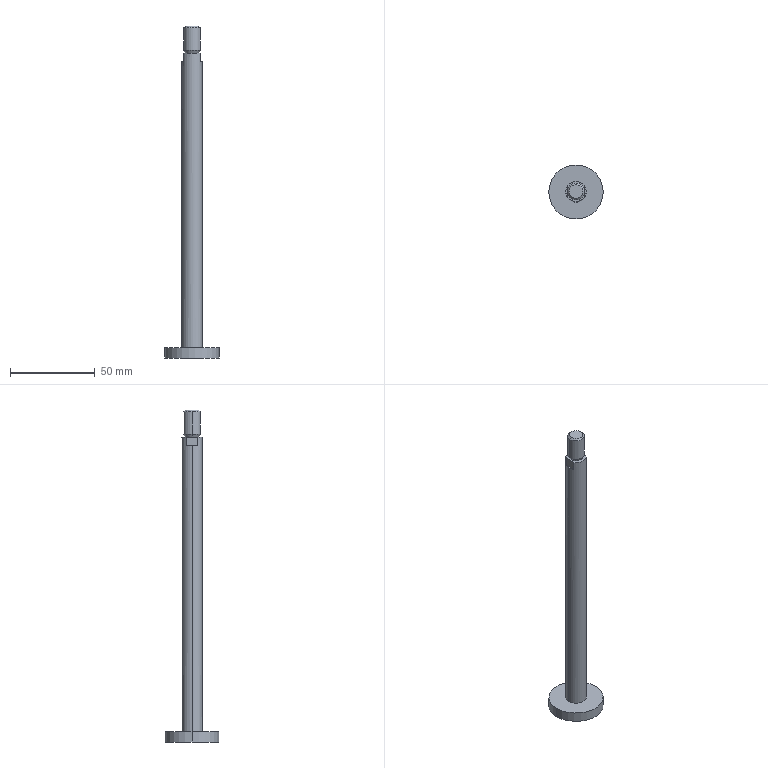Part | STEP file | 1 solid | 18 faces | box 32 x 32 x 195.5 mm | volume 25619 mm3 | plane 8 | cylinder 6 | cone 4 | commonest cylinder face diameters 10 x2 12 x2 32 x2
STEP:
#1=CARTESIAN_POINT('',(0.,0.,0.));
#2=DIRECTION('',(0.,0.,1.));
#3=DIRECTION('',(1.,0.,0.));
#4=AXIS2_PLACEMENT_3D('',#1,#2,#3);
#5=CARTESIAN_POINT('',(16.,0.,-158.5));
#6=VERTEX_POINT('',#5);
#7=CARTESIAN_POINT('',(-16.,0.,-158.5));
#8=VERTEX_POINT('',#7);
#9=CARTESIAN_POINT('',(0.,0.,-158.5));
#10=DIRECTION('',(0.,0.,1.));
#11=DIRECTION('',(1.,0.,0.));
#12=AXIS2_PLACEMENT_3D('',#9,#10,#11);
#13=CIRCLE('',#12,16.);
#14=CARTESIAN_POINT('',(0.,0.,-158.5));
#15=DIRECTION('',(0.,0.,1.));
#16=DIRECTION('',(1.,0.,0.));
#17=AXIS2_PLACEMENT_3D('',#14,#15,#16);
#18=CYLINDRICAL_SURFACE('',#17,16.);
#19=CARTESIAN_POINT('',(0.,0.));
#20=DIRECTION('',(1.,0.));
#21=VECTOR('',#20,1.);
#22=LINE('',#19,#21);
#23=(GEOMETRIC_REPRESENTATION_CONTEXT(2)PARAMETRIC_REPRESENTATION_CONTEXT()REPRESENTATION_CONTEXT('',''));
#24=DEFINITIONAL_REPRESENTATION('',(#22),#23);
#25=PCURVE('',#18,#24);
#26=CARTESIAN_POINT('',(0.,16.,-158.5));
#27=DIRECTION('',(0.,0.,1.));
#28=DIRECTION('',(1.,0.,0.));
#29=AXIS2_PLACEMENT_3D('',#26,#27,#28);
#30=PLANE('',#29);
#31=CARTESIAN_POINT('',(0.,-16.));
#32=DIRECTION('',(1.,0.));
#33=AXIS2_PLACEMENT_2D('',#31,#32);
#34=CIRCLE('',#33,16.);
#35=(GEOMETRIC_REPRESENTATION_CONTEXT(2)PARAMETRIC_REPRESENTATION_CONTEXT()REPRESENTATION_CONTEXT('',''));
#36=DEFINITIONAL_REPRESENTATION('',(#34),#35);
#37=PCURVE('',#30,#36);
#38=SURFACE_CURVE('',#13,(#25,#37),.PCURVE_S1.);
#39=EDGE_CURVE('',#6,#8,#38,.T.);
#40=ORIENTED_EDGE('',*,*,#39,.T.);
#41=CARTESIAN_POINT('',(-16.,0.,-152.5));
#42=VERTEX_POINT('',#41);
#43=CARTESIAN_POINT('',(-16.,0.,-158.5));
#44=DIRECTION('',(0.,0.,1.));
#45=VECTOR('',#44,1.);
#46=LINE('',#43,#45);
#47=CARTESIAN_POINT('',(3.142,0.));
#48=DIRECTION('',(0.,1.));
#49=VECTOR('',#48,1.);
#50=LINE('',#47,#49);
#51=(GEOMETRIC_REPRESENTATION_CONTEXT(2)PARAMETRIC_REPRESENTATION_CONTEXT()REPRESENTATION_CONTEXT('',''));
#52=DEFINITIONAL_REPRESENTATION('',(#50),#51);
#53=PCURVE('',#18,#52);
#54=CARTESIAN_POINT('',(0.,0.,-158.5));
#55=DIRECTION('',(0.,0.,1.));
#56=DIRECTION('',(1.,0.,0.));
#57=AXIS2_PLACEMENT_3D('',#54,#55,#56);
#58=CYLINDRICAL_SURFACE('',#57,16.);
#59=CARTESIAN_POINT('',(3.142,0.));
#60=DIRECTION('',(0.,1.));
#61=VECTOR('',#60,1.);
#62=LINE('',#59,#61);
#63=(GEOMETRIC_REPRESENTATION_CONTEXT(2)PARAMETRIC_REPRESENTATION_CONTEXT()REPRESENTATION_CONTEXT('',''));
#64=DEFINITIONAL_REPRESENTATION('',(#62),#63);
#65=PCURVE('',#58,#64);
#66=SURFACE_CURVE('',#46,(#53,#65),.PCURVE_S1.);
#67=EDGE_CURVE('',#8,#42,#66,.T.);
#68=ORIENTED_EDGE('',*,*,#67,.T.);
#69=CARTESIAN_POINT('',(16.,0.,-152.5));
#70=VERTEX_POINT('',#69);
#71=CARTESIAN_POINT('',(0.,0.,-152.5));
#72=DIRECTION('',(0.,0.,1.));
#73=DIRECTION('',(1.,0.,0.));
#74=AXIS2_PLACEMENT_3D('',#71,#72,#73);
#75=CIRCLE('',#74,16.);
#76=CARTESIAN_POINT('',(0.,6.));
#77=DIRECTION('',(1.,0.));
#78=VECTOR('',#77,1.);
#79=LINE('',#76,#78);
#80=(GEOMETRIC_REPRESENTATION_CONTEXT(2)PARAMETRIC_REPRESENTATION_CONTEXT()REPRESENTATION_CONTEXT('',''));
#81=DEFINITIONAL_REPRESENTATION('',(#79),#80);
#82=PCURVE('',#18,#81);
#83=CARTESIAN_POINT('',(0.,6.,-152.5));
#84=DIRECTION('',(0.,0.,-1.));
#85=DIRECTION('',(-1.,0.,0.));
#86=AXIS2_PLACEMENT_3D('',#83,#84,#85);
#87=PLANE('',#86);
#88=CARTESIAN_POINT('',(-16.,-6.));
#89=CARTESIAN_POINT('',(-16.,21.713));
#90=CARTESIAN_POINT('',(8.,7.856));
#91=CARTESIAN_POINT('',(32.,-6.));
#92=CARTESIAN_POINT('',(8.,-19.856));
#93=CARTESIAN_POINT('',(-16.,-33.713));
#94=CARTESIAN_POINT('',(-16.,-6.));
#95=(BOUNDED_CURVE()B_SPLINE_CURVE(2,(#88,#89,#90,#91,#92,#93,#94),.UNSPECIFIED.,.T.,.F.)B_SPLINE_CURVE_WITH_KNOTS((1,2,2,2,2,1),(-2.094,0.,2.094,4.189,6.283,8.378),.UNSPECIFIED.)CURVE()GEOMETRIC_REPRESENTATION_ITEM()RATIONAL_B_SPLINE_CURVE((1.,0.5,1.,0.5,1.,0.5,1.))REPRESENTATION_ITEM(''));
#96=(GEOMETRIC_REPRESENTATION_CONTEXT(2)PARAMETRIC_REPRESENTATION_CONTEXT()REPRESENTATION_CONTEXT('',''));
#97=DEFINITIONAL_REPRESENTATION('',(#95),#96);
#98=PCURVE('',#87,#97);
#99=SURFACE_CURVE('',#75,(#82,#98),.PCURVE_S1.);
#100=EDGE_CURVE('',#70,#42,#99,.T.);
#101=ORIENTED_EDGE('',*,*,#100,.F.);
#102=CARTESIAN_POINT('',(16.,0.,-158.5));
#103=DIRECTION('',(0.,0.,1.));
#104=VECTOR('',#103,1.);
#105=LINE('',#102,#104);
#106=CARTESIAN_POINT('',(0.,0.));
#107=DIRECTION('',(0.,1.));
#108=VECTOR('',#107,1.);
#109=LINE('',#106,#108);
#110=(GEOMETRIC_REPRESENTATION_CONTEXT(2)PARAMETRIC_REPRESENTATION_CONTEXT()REPRESENTATION_CONTEXT('',''));
#111=DEFINITIONAL_REPRESENTATION('',(#109),#110);
#112=PCURVE('',#18,#111);
#113=CARTESIAN_POINT('',(6.283,0.));
#114=DIRECTION('',(0.,1.));
#115=VECTOR('',#114,1.);
#116=LINE('',#113,#115);
#117=(GEOMETRIC_REPRESENTATION_CONTEXT(2)PARAMETRIC_REPRESENTATION_CONTEXT()REPRESENTATION_CONTEXT('',''));
#118=DEFINITIONAL_REPRESENTATION('',(#116),#117);
#119=PCURVE('',#58,#118);
#120=SURFACE_CURVE('',#105,(#112,#119),.PCURVE_S1.);
#121=EDGE_CURVE('',#6,#70,#120,.T.);
#122=ORIENTED_EDGE('',*,*,#121,.F.);
#123=EDGE_LOOP('',(#40,#68,#101,#122));
#124=FACE_BOUND('',#123,.T.);
#125=ADVANCED_FACE('',(#124),#18,.T.);
#126=CARTESIAN_POINT('',(6.,0.,-152.5));
#127=VERTEX_POINT('',#126);
#128=CARTESIAN_POINT('',(-6.,0.,-152.5));
#129=VERTEX_POINT('',#128);
#130=CARTESIAN_POINT('',(0.,0.,-152.5));
#131=DIRECTION('',(0.,0.,1.));
#132=DIRECTION('',(1.,0.,0.));
#133=AXIS2_PLACEMENT_3D('',#130,#131,#132);
#134=CIRCLE('',#133,6.);
#135=CARTESIAN_POINT('',(0.,0.,-158.5));
#136=DIRECTION('',(0.,0.,1.));
#137=DIRECTION('',(1.,0.,0.));
#138=AXIS2_PLACEMENT_3D('',#135,#136,#137);
#139=CYLINDRICAL_SURFACE('',#138,6.);
#140=CARTESIAN_POINT('',(0.,6.));
#141=DIRECTION('',(1.,0.));
#142=VECTOR('',#141,1.);
#143=LINE('',#140,#142);
#144=(GEOMETRIC_REPRESENTATION_CONTEXT(2)PARAMETRIC_REPRESENTATION_CONTEXT()REPRESENTATION_CONTEXT('',''));
#145=DEFINITIONAL_REPRESENTATION('',(#143),#144);
#146=PCURVE('',#139,#145);
#147=CARTESIAN_POINT('',(-6.,-6.));
#148=CARTESIAN_POINT('',(-6.,4.392));
#149=CARTESIAN_POINT('',(3.,-0.8038));
#150=CARTESIAN_POINT('',(12.,-6.));
#151=CARTESIAN_POINT('',(3.,-11.196));
#152=CARTESIAN_POINT('',(-6.,-16.392));
#153=CARTESIAN_POINT('',(-6.,-6.));
#154=(BOUNDED_CURVE()B_SPLINE_CURVE(2,(#147,#148,#149,#150,#151,#152,#153),.UNSPECIFIED.,.T.,.F.)B_SPLINE_CURVE_WITH_KNOTS((1,2,2,2,2,1),(-2.094,0.,2.094,4.189,6.283,8.378),.UNSPECIFIED.)CURVE()GEOMETRIC_REPRESENTATION_ITEM()RATIONAL_B_SPLINE_CURVE((1.,0.5,1.,0.5,1.,0.5,1.))REPRESENTATION_ITEM(''));
#155=(GEOMETRIC_REPRESENTATION_CONTEXT(2)PARAMETRIC_REPRESENTATION_CONTEXT()REPRESENTATION_CONTEXT('',''));
#156=DEFINITIONAL_REPRESENTATION('',(#154),#155);
#157=PCURVE('',#87,#156);
#158=SURFACE_CURVE('',#134,(#146,#157),.PCURVE_S1.);
#159=EDGE_CURVE('',#127,#129,#158,.T.);
#160=ORIENTED_EDGE('',*,*,#159,.T.);
#161=CARTESIAN_POINT('',(-6.,0.,16.));
#162=VERTEX_POINT('',#161);
#163=CARTESIAN_POINT('',(-6.,0.,-158.5));
#164=DIRECTION('',(0.,0.,1.));
#165=VECTOR('',#164,1.);
#166=LINE('',#163,#165);
#167=CARTESIAN_POINT('',(3.142,0.));
#168=DIRECTION('',(0.,1.));
#169=VECTOR('',#168,1.);
#170=LINE('',#167,#169);
#171=(GEOMETRIC_REPRESENTATION_CONTEXT(2)PARAMETRIC_REPRESENTATION_CONTEXT()REPRESENTATION_CONTEXT('',''));
#172=DEFINITIONAL_REPRESENTATION('',(#170),#171);
#173=PCURVE('',#139,#172);
#174=CARTESIAN_POINT('',(0.,0.,-158.5));
#175=DIRECTION('',(0.,0.,1.));
#176=DIRECTION('',(1.,0.,0.));
#177=AXIS2_PLACEMENT_3D('',#174,#175,#176);
#178=CYLINDRICAL_SURFACE('',#177,6.);
#179=CARTESIAN_POINT('',(3.142,0.));
#180=DIRECTION('',(0.,1.));
#181=VECTOR('',#180,1.);
#182=LINE('',#179,#181);
#183=(GEOMETRIC_REPRESENTATION_CONTEXT(2)PARAMETRIC_REPRESENTATION_CONTEXT()REPRESENTATION_CONTEXT('',''));
#184=DEFINITIONAL_REPRESENTATION('',(#182),#183);
#185=PCURVE('',#178,#184);
#186=SURFACE_CURVE('',#166,(#173,#185),.PCURVE_S1.);
#187=EDGE_CURVE('',#129,#162,#186,.T.);
#188=ORIENTED_EDGE('',*,*,#187,.T.);
#189=CARTESIAN_POINT('',(-5.,3.317,16.));
#190=VERTEX_POINT('',#189);
#191=CARTESIAN_POINT('',(0.,0.,16.));
#192=DIRECTION('',(0.,0.,-1.));
#193=DIRECTION('',(-1.,0.,0.));
#194=AXIS2_PLACEMENT_3D('',#191,#192,#193);
#195=CIRCLE('',#194,6.);
#196=CARTESIAN_POINT('',(3.142,174.5));
#197=DIRECTION('',(-1.,0.));
#198=VECTOR('',#197,1.);
#199=LINE('',#196,#198);
#200=(GEOMETRIC_REPRESENTATION_CONTEXT(2)PARAMETRIC_REPRESENTATION_CONTEXT()REPRESENTATION_CONTEXT('',''));
#201=DEFINITIONAL_REPRESENTATION('',(#199),#200);
#202=PCURVE('',#139,#201);
#203=CARTESIAN_POINT('',(-5.,-12.,16.));
#204=DIRECTION('',(0.,0.,-1.));
#205=DIRECTION('',(-1.,0.,0.));
#206=AXIS2_PLACEMENT_3D('',#203,#204,#205);
#207=PLANE('',#206);
#208=CARTESIAN_POINT('',(-5.,12.));
#209=DIRECTION('',(1.,0.));
#210=AXIS2_PLACEMENT_2D('',#208,#209);
#211=CIRCLE('',#210,6.);
#212=(GEOMETRIC_REPRESENTATION_CONTEXT(2)PARAMETRIC_REPRESENTATION_CONTEXT()REPRESENTATION_CONTEXT('',''));
#213=DEFINITIONAL_REPRESENTATION('',(#211),#212);
#214=PCURVE('',#207,#213);
#215=SURFACE_CURVE('',#195,(#202,#214),.PCURVE_S1.);
#216=EDGE_CURVE('',#162,#190,#215,.T.);
#217=ORIENTED_EDGE('',*,*,#216,.T.);
#218=CARTESIAN_POINT('',(-5.,3.317,21.));
#219=VERTEX_POINT('',#218);
#220=CARTESIAN_POINT('',(-5.,3.317,-158.5));
#221=DIRECTION('',(0.,0.,1.));
#222=VECTOR('',#221,1.);
#223=LINE('',#220,#222);
#224=CARTESIAN_POINT('',(2.556,0.));
#225=DIRECTION('',(0.,1.));
#226=VECTOR('',#225,1.);
#227=LINE('',#224,#226);
#228=(GEOMETRIC_REPRESENTATION_CONTEXT(2)PARAMETRIC_REPRESENTATION_CONTEXT()REPRESENTATION_CONTEXT('',''));
#229=DEFINITIONAL_REPRESENTATION('',(#227),#228);
#230=PCURVE('',#139,#229);
#231=CARTESIAN_POINT('',(-5.,-12.,21.));
#232=DIRECTION('',(1.,0.,0.));
#233=DIRECTION('',(0.,0.,-1.));
#234=AXIS2_PLACEMENT_3D('',#231,#232,#233);
#235=PLANE('',#234);
#236=CARTESIAN_POINT('',(179.5,15.317));
#237=DIRECTION('',(-1.,0.));
#238=VECTOR('',#237,1.);
#239=LINE('',#236,#238);
#240=(GEOMETRIC_REPRESENTATION_CONTEXT(2)PARAMETRIC_REPRESENTATION_CONTEXT()REPRESENTATION_CONTEXT('',''));
#241=DEFINITIONAL_REPRESENTATION('',(#239),#240);
#242=PCURVE('',#235,#241);
#243=SURFACE_CURVE('',#223,(#230,#242),.PCURVE_S1.);
#244=EDGE_CURVE('',#190,#219,#243,.T.);
#245=ORIENTED_EDGE('',*,*,#244,.T.);
#246=CARTESIAN_POINT('',(5.,3.317,21.));
#247=VERTEX_POINT('',#246);
#248=CARTESIAN_POINT('',(0.,0.,21.));
#249=DIRECTION('',(0.,0.,1.));
#250=DIRECTION('',(1.,0.,0.));
#251=AXIS2_PLACEMENT_3D('',#248,#249,#250);
#252=CIRCLE('',#251,6.);
#253=CARTESIAN_POINT('',(0.,179.5));
#254=DIRECTION('',(1.,0.));
#255=VECTOR('',#254,1.);
#256=LINE('',#253,#255);
#257=(GEOMETRIC_REPRESENTATION_CONTEXT(2)PARAMETRIC_REPRESENTATION_CONTEXT()REPRESENTATION_CONTEXT('',''));
#258=DEFINITIONAL_REPRESENTATION('',(#256),#257);
#259=PCURVE('',#139,#258);
#260=CARTESIAN_POINT('',(0.,4.,21.));
#261=DIRECTION('',(0.,0.,-1.));
#262=DIRECTION('',(-1.,0.,0.));
#263=AXIS2_PLACEMENT_3D('',#260,#261,#262);
#264=PLANE('',#263);
#265=CARTESIAN_POINT('',(-6.,-4.));
#266=CARTESIAN_POINT('',(-6.,6.392));
#267=CARTESIAN_POINT('',(3.,1.196));
#268=CARTESIAN_POINT('',(12.,-4.));
#269=CARTESIAN_POINT('',(3.,-9.196));
#270=CARTESIAN_POINT('',(-6.,-14.392));
#271=CARTESIAN_POINT('',(-6.,-4.));
#272=(BOUNDED_CURVE()B_SPLINE_CURVE(2,(#265,#266,#267,#268,#269,#270,#271),.UNSPECIFIED.,.T.,.F.)B_SPLINE_CURVE_WITH_KNOTS((1,2,2,2,2,1),(-2.094,0.,2.094,4.189,6.283,8.378),.UNSPECIFIED.)CURVE()GEOMETRIC_REPRESENTATION_ITEM()RATIONAL_B_SPLINE_CURVE((1.,0.5,1.,0.5,1.,0.5,1.))REPRESENTATION_ITEM(''));
#273=(GEOMETRIC_REPRESENTATION_CONTEXT(2)PARAMETRIC_REPRESENTATION_CONTEXT()REPRESENTATION_CONTEXT('',''));
#274=DEFINITIONAL_REPRESENTATION('',(#272),#273);
#275=PCURVE('',#264,#274);
#276=SURFACE_CURVE('',#252,(#259,#275),.PCURVE_S1.);
#277=EDGE_CURVE('',#247,#219,#276,.T.);
#278=ORIENTED_EDGE('',*,*,#277,.F.);
#279=CARTESIAN_POINT('',(5.,3.317,16.));
#280=VERTEX_POINT('',#279);
#281=CARTESIAN_POINT('',(5.,3.317,-158.5));
#282=DIRECTION('',(0.,0.,-1.));
#283=VECTOR('',#282,1.);
#284=LINE('',#281,#283);
#285=CARTESIAN_POINT('',(0.5857,0.));
#286=DIRECTION('',(0.,-1.));
#287=VECTOR('',#286,1.);
#288=LINE('',#285,#287);
#289=(GEOMETRIC_REPRESENTATION_CONTEXT(2)PARAMETRIC_REPRESENTATION_CONTEXT()REPRESENTATION_CONTEXT('',''));
#290=DEFINITIONAL_REPRESENTATION('',(#288),#289);
#291=PCURVE('',#139,#290);
#292=CARTESIAN_POINT('',(5.,-12.,16.));
#293=DIRECTION('',(-1.,0.,0.));
#294=DIRECTION('',(0.,0.,1.));
#295=AXIS2_PLACEMENT_3D('',#292,#293,#294);
#296=PLANE('',#295);
#297=CARTESIAN_POINT('',(-174.5,15.317));
#298=DIRECTION('',(-1.,0.));
#299=VECTOR('',#298,1.);
#300=LINE('',#297,#299);
#301=(GEOMETRIC_REPRESENTATION_CONTEXT(2)PARAMETRIC_REPRESENTATION_CONTEXT()REPRESENTATION_CONTEXT('',''));
#302=DEFINITIONAL_REPRESENTATION('',(#300),#301);
#303=PCURVE('',#296,#302);
#304=SURFACE_CURVE('',#284,(#291,#303),.PCURVE_S1.);
#305=EDGE_CURVE('',#247,#280,#304,.T.);
#306=ORIENTED_EDGE('',*,*,#305,.T.);
#307=CARTESIAN_POINT('',(6.,0.,16.));
#308=VERTEX_POINT('',#307);
#309=CARTESIAN_POINT('',(0.,0.,16.));
#310=DIRECTION('',(0.,0.,-1.));
#311=DIRECTION('',(-1.,0.,0.));
#312=AXIS2_PLACEMENT_3D('',#309,#310,#311);
#313=CIRCLE('',#312,6.);
#314=CARTESIAN_POINT('',(3.142,174.5));
#315=DIRECTION('',(-1.,0.));
#316=VECTOR('',#315,1.);
#317=LINE('',#314,#316);
#318=(GEOMETRIC_REPRESENTATION_CONTEXT(2)PARAMETRIC_REPRESENTATION_CONTEXT()REPRESENTATION_CONTEXT('',''));
#319=DEFINITIONAL_REPRESENTATION('',(#317),#318);
#320=PCURVE('',#139,#319);
#321=CARTESIAN_POINT('',(17.,-12.,16.));
#322=DIRECTION('',(0.,0.,-1.));
#323=DIRECTION('',(-1.,0.,0.));
#324=AXIS2_PLACEMENT_3D('',#321,#322,#323);
#325=PLANE('',#324);
#326=CARTESIAN_POINT('',(17.,12.));
#327=DIRECTION('',(1.,0.));
#328=AXIS2_PLACEMENT_2D('',#326,#327);
#329=CIRCLE('',#328,6.);
#330=(GEOMETRIC_REPRESENTATION_CONTEXT(2)PARAMETRIC_REPRESENTATION_CONTEXT()REPRESENTATION_CONTEXT('',''));
#331=DEFINITIONAL_REPRESENTATION('',(#329),#330);
#332=PCURVE('',#325,#331);
#333=SURFACE_CURVE('',#313,(#320,#332),.PCURVE_S1.);
#334=EDGE_CURVE('',#280,#308,#333,.T.);
#335=ORIENTED_EDGE('',*,*,#334,.T.);
#336=CARTESIAN_POINT('',(6.,0.,-158.5));
#337=DIRECTION('',(0.,0.,1.));
#338=VECTOR('',#337,1.);
#339=LINE('',#336,#338);
#340=CARTESIAN_POINT('',(0.,0.));
#341=DIRECTION('',(0.,1.));
#342=VECTOR('',#341,1.);
#343=LINE('',#340,#342);
#344=(GEOMETRIC_REPRESENTATION_CONTEXT(2)PARAMETRIC_REPRESENTATION_CONTEXT()REPRESENTATION_CONTEXT('',''));
#345=DEFINITIONAL_REPRESENTATION('',(#343),#344);
#346=PCURVE('',#139,#345);
#347=CARTESIAN_POINT('',(6.283,0.));
#348=DIRECTION('',(0.,1.));
#349=VECTOR('',#348,1.);
#350=LINE('',#347,#349);
#351=(GEOMETRIC_REPRESENTATION_CONTEXT(2)PARAMETRIC_REPRESENTATION_CONTEXT()REPRESENTATION_CONTEXT('',''));
#352=DEFINITIONAL_REPRESENTATION('',(#350),#351);
#353=PCURVE('',#178,#352);
#354=SURFACE_CURVE('',#339,(#346,#353),.PCURVE_S1.);
#355=EDGE_CURVE('',#127,#308,#354,.T.);
#356=ORIENTED_EDGE('',*,*,#355,.F.);
#357=EDGE_LOOP('',(#160,#188,#217,#245,#278,#306,#335,#356));
#358=FACE_BOUND('',#357,.T.);
#359=ADVANCED_FACE('',(#358),#139,.T.);
#360=CARTESIAN_POINT('',(4.,0.,21.));
#361=VERTEX_POINT('',#360);
#362=CARTESIAN_POINT('',(-4.,0.,21.));
#363=VERTEX_POINT('',#362);
#364=CARTESIAN_POINT('',(0.,0.,21.));
#365=DIRECTION('',(0.,0.,1.));
#366=DIRECTION('',(1.,0.,0.));
#367=AXIS2_PLACEMENT_3D('',#364,#365,#366);
#368=CIRCLE('',#367,4.);
#369=CARTESIAN_POINT('',(0.,0.,21.));
#370=DIRECTION('',(0.,0.,1.));
#371=DIRECTION('',(1.,0.,0.));
#372=AXIS2_PLACEMENT_3D('',#369,#370,#371);
#373=CONICAL_SURFACE('',#372,4.,0.5236);
#374=CARTESIAN_POINT('',(0.,0.));
#375=DIRECTION('',(1.,0.));
#376=VECTOR('',#375,1.);
#377=LINE('',#374,#376);
#378=(GEOMETRIC_REPRESENTATION_CONTEXT(2)PARAMETRIC_REPRESENTATION_CONTEXT()REPRESENTATION_CONTEXT('',''));
#379=DEFINITIONAL_REPRESENTATION('',(#377),#378);
#380=PCURVE('',#373,#379);
#381=CARTESIAN_POINT('',(-4.,-4.));
#382=CARTESIAN_POINT('',(-4.,2.928));
#383=CARTESIAN_POINT('',(2.,-0.5359));
#384=CARTESIAN_POINT('',(8.,-4.));
#385=CARTESIAN_POINT('',(2.,-7.464));
#386=CARTESIAN_POINT('',(-4.,-10.928));
#387=CARTESIAN_POINT('',(-4.,-4.));
#388=(BOUNDED_CURVE()B_SPLINE_CURVE(2,(#381,#382,#383,#384,#385,#386,#387),.UNSPECIFIED.,.T.,.F.)B_SPLINE_CURVE_WITH_KNOTS((1,2,2,2,2,1),(-2.094,0.,2.094,4.189,6.283,8.378),.UNSPECIFIED.)CURVE()GEOMETRIC_REPRESENTATION_ITEM()RATIONAL_B_SPLINE_CURVE((1.,0.5,1.,0.5,1.,0.5,1.))REPRESENTATION_ITEM(''));
#389=(GEOMETRIC_REPRESENTATION_CONTEXT(2)PARAMETRIC_REPRESENTATION_CONTEXT()REPRESENTATION_CONTEXT('',''));
#390=DEFINITIONAL_REPRESENTATION('',(#388),#389);
#391=PCURVE('',#264,#390);
#392=SURFACE_CURVE('',#368,(#380,#391),.PCURVE_S1.);
#393=EDGE_CURVE('',#361,#363,#392,.T.);
#394=ORIENTED_EDGE('',*,*,#393,.T.);
#395=CARTESIAN_POINT('',(-5.,0.,22.732));
#396=VERTEX_POINT('',#395);
#397=CARTESIAN_POINT('',(-4.,0.,21.));
#398=DIRECTION('',(-0.5,0.,0.866));
#399=VECTOR('',#398,1.);
#400=LINE('',#397,#399);
#401=CARTESIAN_POINT('',(3.142,0.));
#402=DIRECTION('',(0.,1.));
#403=VECTOR('',#402,1.);
#404=LINE('',#401,#403);
#405=(GEOMETRIC_REPRESENTATION_CONTEXT(2)PARAMETRIC_REPRESENTATION_CONTEXT()REPRESENTATION_CONTEXT('',''));
#406=DEFINITIONAL_REPRESENTATION('',(#404),#405);
#407=PCURVE('',#373,#406);
#408=CARTESIAN_POINT('',(0.,0.,21.));
#409=DIRECTION('',(0.,0.,1.));
#410=DIRECTION('',(1.,0.,0.));
#411=AXIS2_PLACEMENT_3D('',#408,#409,#410);
#412=CONICAL_SURFACE('',#411,4.,0.5236);
#413=CARTESIAN_POINT('',(3.142,0.));
#414=DIRECTION('',(0.,1.));
#415=VECTOR('',#414,1.);
#416=LINE('',#413,#415);
#417=(GEOMETRIC_REPRESENTATION_CONTEXT(2)PARAMETRIC_REPRESENTATION_CONTEXT()REPRESENTATION_CONTEXT('',''));
#418=DEFINITIONAL_REPRESENTATION('',(#416),#417);
#419=PCURVE('',#412,#418);
#420=SURFACE_CURVE('',#400,(#407,#419),.PCURVE_S1.);
#421=EDGE_CURVE('',#363,#396,#420,.T.);
#422=ORIENTED_EDGE('',*,*,#421,.T.);
#423=CARTESIAN_POINT('',(5.,0.,22.732));
#424=VERTEX_POINT('',#423);
#425=CARTESIAN_POINT('',(0.,0.,22.732));
#426=DIRECTION('',(0.,0.,1.));
#427=DIRECTION('',(1.,0.,0.));
#428=AXIS2_PLACEMENT_3D('',#425,#426,#427);
#429=CIRCLE('',#428,5.);
#430=CARTESIAN_POINT('',(0.,1.732));
#431=DIRECTION('',(1.,0.));
#432=VECTOR('',#431,1.);
#433=LINE('',#430,#432);
#434=(GEOMETRIC_REPRESENTATION_CONTEXT(2)PARAMETRIC_REPRESENTATION_CONTEXT()REPRESENTATION_CONTEXT('',''));
#435=DEFINITIONAL_REPRESENTATION('',(#433),#434);
#436=PCURVE('',#373,#435);
#437=CARTESIAN_POINT('',(0.,0.,-158.5));
#438=DIRECTION('',(0.,0.,1.));
#439=DIRECTION('',(1.,0.,0.));
#440=AXIS2_PLACEMENT_3D('',#437,#438,#439);
#441=CYLINDRICAL_SURFACE('',#440,5.);
#442=CARTESIAN_POINT('',(0.,181.232));
#443=DIRECTION('',(1.,0.));
#444=VECTOR('',#443,1.);
#445=LINE('',#442,#444);
#446=(GEOMETRIC_REPRESENTATION_CONTEXT(2)PARAMETRIC_REPRESENTATION_CONTEXT()REPRESENTATION_CONTEXT('',''));
#447=DEFINITIONAL_REPRESENTATION('',(#445),#446);
#448=PCURVE('',#441,#447);
#449=SURFACE_CURVE('',#429,(#436,#448),.PCURVE_S1.);
#450=EDGE_CURVE('',#424,#396,#449,.T.);
#451=ORIENTED_EDGE('',*,*,#450,.F.);
#452=CARTESIAN_POINT('',(4.,0.,21.));
#453=DIRECTION('',(0.5,0.,0.866));
#454=VECTOR('',#453,1.);
#455=LINE('',#452,#454);
#456=CARTESIAN_POINT('',(0.,0.));
#457=DIRECTION('',(0.,1.));
#458=VECTOR('',#457,1.);
#459=LINE('',#456,#458);
#460=(GEOMETRIC_REPRESENTATION_CONTEXT(2)PARAMETRIC_REPRESENTATION_CONTEXT()REPRESENTATION_CONTEXT('',''));
#461=DEFINITIONAL_REPRESENTATION('',(#459),#460);
#462=PCURVE('',#373,#461);
#463=CARTESIAN_POINT('',(6.283,0.));
#464=DIRECTION('',(0.,1.));
#465=VECTOR('',#464,1.);
#466=LINE('',#463,#465);
#467=(GEOMETRIC_REPRESENTATION_CONTEXT(2)PARAMETRIC_REPRESENTATION_CONTEXT()REPRESENTATION_CONTEXT('',''));
#468=DEFINITIONAL_REPRESENTATION('',(#466),#467);
#469=PCURVE('',#412,#468);
#470=SURFACE_CURVE('',#455,(#462,#469),.PCURVE_S1.);
#471=EDGE_CURVE('',#361,#424,#470,.T.);
#472=ORIENTED_EDGE('',*,*,#471,.F.);
#473=EDGE_LOOP('',(#394,#422,#451,#472));
#474=FACE_BOUND('',#473,.T.);
#475=ADVANCED_FACE('',(#474),#373,.T.);
#476=ORIENTED_EDGE('',*,*,#450,.T.);
#477=CARTESIAN_POINT('',(-5.,0.,36.));
#478=VERTEX_POINT('',#477);
#479=CARTESIAN_POINT('',(-5.,0.,-158.5));
#480=DIRECTION('',(0.,0.,1.));
#481=VECTOR('',#480,1.);
#482=LINE('',#479,#481);
#483=CARTESIAN_POINT('',(3.142,0.));
#484=DIRECTION('',(0.,1.));
#485=VECTOR('',#484,1.);
#486=LINE('',#483,#485);
#487=(GEOMETRIC_REPRESENTATION_CONTEXT(2)PARAMETRIC_REPRESENTATION_CONTEXT()REPRESENTATION_CONTEXT('',''));
#488=DEFINITIONAL_REPRESENTATION('',(#486),#487);
#489=PCURVE('',#441,#488);
#490=CARTESIAN_POINT('',(0.,0.,-158.5));
#491=DIRECTION('',(0.,0.,1.));
#492=DIRECTION('',(1.,0.,0.));
#493=AXIS2_PLACEMENT_3D('',#490,#491,#492);
#494=CYLINDRICAL_SURFACE('',#493,5.);
#495=CARTESIAN_POINT('',(3.142,0.));
#496=DIRECTION('',(0.,1.));
#497=VECTOR('',#496,1.);
#498=LINE('',#495,#497);
#499=(GEOMETRIC_REPRESENTATION_CONTEXT(2)PARAMETRIC_REPRESENTATION_CONTEXT()REPRESENTATION_CONTEXT('',''));
#500=DEFINITIONAL_REPRESENTATION('',(#498),#499);
#501=PCURVE('',#494,#500);
#502=SURFACE_CURVE('',#482,(#489,#501),.PCURVE_S1.);
#503=EDGE_CURVE('',#396,#478,#502,.T.);
#504=ORIENTED_EDGE('',*,*,#503,.T.);
#505=CARTESIAN_POINT('',(5.,0.,36.));
#506=VERTEX_POINT('',#505);
#507=CARTESIAN_POINT('',(0.,0.,36.));
#508=DIRECTION('',(0.,0.,1.));
#509=DIRECTION('',(1.,0.,0.));
#510=AXIS2_PLACEMENT_3D('',#507,#508,#509);
#511=CIRCLE('',#510,5.);
#512=CARTESIAN_POINT('',(0.,194.5));
#513=DIRECTION('',(1.,0.));
#514=VECTOR('',#513,1.);
#515=LINE('',#512,#514);
#516=(GEOMETRIC_REPRESENTATION_CONTEXT(2)PARAMETRIC_REPRESENTATION_CONTEXT()REPRESENTATION_CONTEXT('',''));
#517=DEFINITIONAL_REPRESENTATION('',(#515),#516);
#518=PCURVE('',#441,#517);
#519=CARTESIAN_POINT('',(0.,0.,36.));
#520=DIRECTION('',(0.,0.,-1.));
#521=DIRECTION('',(-1.,0.,0.));
#522=AXIS2_PLACEMENT_3D('',#519,#520,#521);
#523=CONICAL_SURFACE('',#522,5.,0.7854);
#524=CARTESIAN_POINT('',(3.142,0.));
#525=DIRECTION('',(-1.,0.));
#526=VECTOR('',#525,1.);
#527=LINE('',#524,#526);
#528=(GEOMETRIC_REPRESENTATION_CONTEXT(2)PARAMETRIC_REPRESENTATION_CONTEXT()REPRESENTATION_CONTEXT('',''));
#529=DEFINITIONAL_REPRESENTATION('',(#527),#528);
#530=PCURVE('',#523,#529);
#531=SURFACE_CURVE('',#511,(#518,#530),.PCURVE_S1.);
#532=EDGE_CURVE('',#506,#478,#531,.T.);
#533=ORIENTED_EDGE('',*,*,#532,.F.);
#534=CARTESIAN_POINT('',(5.,0.,-158.5));
#535=DIRECTION('',(0.,0.,1.));
#536=VECTOR('',#535,1.);
#537=LINE('',#534,#536);
#538=CARTESIAN_POINT('',(0.,0.));
#539=DIRECTION('',(0.,1.));
#540=VECTOR('',#539,1.);
#541=LINE('',#538,#540);
#542=(GEOMETRIC_REPRESENTATION_CONTEXT(2)PARAMETRIC_REPRESENTATION_CONTEXT()REPRESENTATION_CONTEXT('',''));
#543=DEFINITIONAL_REPRESENTATION('',(#541),#542);
#544=PCURVE('',#441,#543);
#545=CARTESIAN_POINT('',(6.283,0.));
#546=DIRECTION('',(0.,1.));
#547=VECTOR('',#546,1.);
#548=LINE('',#545,#547);
#549=(GEOMETRIC_REPRESENTATION_CONTEXT(2)PARAMETRIC_REPRESENTATION_CONTEXT()REPRESENTATION_CONTEXT('',''));
#550=DEFINITIONAL_REPRESENTATION('',(#548),#549);
#551=PCURVE('',#494,#550);
#552=SURFACE_CURVE('',#537,(#544,#551),.PCURVE_S1.);
#553=EDGE_CURVE('',#424,#506,#552,.T.);
#554=ORIENTED_EDGE('',*,*,#553,.F.);
#555=EDGE_LOOP('',(#476,#504,#533,#554));
#556=FACE_BOUND('',#555,.T.);
#557=ADVANCED_FACE('',(#556),#441,.T.);
#558=CARTESIAN_POINT('',(4.,0.,37.));
#559=VERTEX_POINT('',#558);
#560=CARTESIAN_POINT('',(-4.,0.,37.));
#561=VERTEX_POINT('',#560);
#562=CARTESIAN_POINT('',(0.,0.,37.));
#563=DIRECTION('',(0.,0.,1.));
#564=DIRECTION('',(1.,0.,0.));
#565=AXIS2_PLACEMENT_3D('',#562,#563,#564);
#566=CIRCLE('',#565,4.);
#567=CARTESIAN_POINT('',(3.142,-1.));
#568=DIRECTION('',(-1.,0.));
#569=VECTOR('',#568,1.);
#570=LINE('',#567,#569);
#571=(GEOMETRIC_REPRESENTATION_CONTEXT(2)PARAMETRIC_REPRESENTATION_CONTEXT()REPRESENTATION_CONTEXT('',''));
#572=DEFINITIONAL_REPRESENTATION('',(#570),#571);
#573=PCURVE('',#523,#572);
#574=CARTESIAN_POINT('',(0.,0.,37.));
#575=DIRECTION('',(0.,0.,-1.));
#576=DIRECTION('',(-1.,0.,0.));
#577=AXIS2_PLACEMENT_3D('',#574,#575,#576);
#578=PLANE('',#577);
#579=CARTESIAN_POINT('',(-4.,0.));
#580=CARTESIAN_POINT('',(-4.,6.928));
#581=CARTESIAN_POINT('',(2.,3.464));
#582=CARTESIAN_POINT('',(8.,0.));
#583=CARTESIAN_POINT('',(2.,-3.464));
#584=CARTESIAN_POINT('',(-4.,-6.928));
#585=CARTESIAN_POINT('',(-4.,0.));
#586=(BOUNDED_CURVE()B_SPLINE_CURVE(2,(#579,#580,#581,#582,#583,#584,#585),.UNSPECIFIED.,.T.,.F.)B_SPLINE_CURVE_WITH_KNOTS((1,2,2,2,2,1),(-2.094,0.,2.094,4.189,6.283,8.378),.UNSPECIFIED.)CURVE()GEOMETRIC_REPRESENTATION_ITEM()RATIONAL_B_SPLINE_CURVE((1.,0.5,1.,0.5,1.,0.5,1.))REPRESENTATION_ITEM(''));
#587=(GEOMETRIC_REPRESENTATION_CONTEXT(2)PARAMETRIC_REPRESENTATION_CONTEXT()REPRESENTATION_CONTEXT('',''));
#588=DEFINITIONAL_REPRESENTATION('',(#586),#587);
#589=PCURVE('',#578,#588);
#590=SURFACE_CURVE('',#566,(#573,#589),.PCURVE_S1.);
#591=EDGE_CURVE('',#559,#561,#590,.T.);
#592=ORIENTED_EDGE('',*,*,#591,.F.);
#593=CARTESIAN_POINT('',(5.,0.,36.));
#594=DIRECTION('',(0.7071,0.,-0.7071));
#595=VECTOR('',#594,1.);
#596=LINE('',#593,#595);
#597=CARTESIAN_POINT('',(3.142,0.));
#598=DIRECTION('',(0.,1.));
#599=VECTOR('',#598,1.);
#600=LINE('',#597,#599);
#601=(GEOMETRIC_REPRESENTATION_CONTEXT(2)PARAMETRIC_REPRESENTATION_CONTEXT()REPRESENTATION_CONTEXT('',''));
#602=DEFINITIONAL_REPRESENTATION('',(#600),#601);
#603=PCURVE('',#523,#602);
#604=CARTESIAN_POINT('',(0.,0.,36.));
#605=DIRECTION('',(0.,0.,-1.));
#606=DIRECTION('',(-1.,0.,0.));
#607=AXIS2_PLACEMENT_3D('',#604,#605,#606);
#608=CONICAL_SURFACE('',#607,5.,0.7854);
#609=CARTESIAN_POINT('',(3.142,0.));
#610=DIRECTION('',(0.,1.));
#611=VECTOR('',#610,1.);
#612=LINE('',#609,#611);
#613=(GEOMETRIC_REPRESENTATION_CONTEXT(2)PARAMETRIC_REPRESENTATION_CONTEXT()REPRESENTATION_CONTEXT('',''));
#614=DEFINITIONAL_REPRESENTATION('',(#612),#613);
#615=PCURVE('',#608,#614);
#616=SURFACE_CURVE('',#596,(#603,#615),.PCURVE_S1.);
#617=EDGE_CURVE('',#559,#506,#616,.T.);
#618=ORIENTED_EDGE('',*,*,#617,.T.);
#619=ORIENTED_EDGE('',*,*,#532,.T.);
#620=CARTESIAN_POINT('',(-5.,0.,36.));
#621=DIRECTION('',(-0.7071,0.,-0.7071));
#622=VECTOR('',#621,1.);
#623=LINE('',#620,#622);
#624=CARTESIAN_POINT('',(0.,0.));
#625=DIRECTION('',(0.,1.));
#626=VECTOR('',#625,1.);
#627=LINE('',#624,#626);
#628=(GEOMETRIC_REPRESENTATION_CONTEXT(2)PARAMETRIC_REPRESENTATION_CONTEXT()REPRESENTATION_CONTEXT('',''));
#629=DEFINITIONAL_REPRESENTATION('',(#627),#628);
#630=PCURVE('',#523,#629);
#631=CARTESIAN_POINT('',(6.283,0.));
#632=DIRECTION('',(0.,1.));
#633=VECTOR('',#632,1.);
#634=LINE('',#631,#633);
#635=(GEOMETRIC_REPRESENTATION_CONTEXT(2)PARAMETRIC_REPRESENTATION_CONTEXT()REPRESENTATION_CONTEXT('',''));
#636=DEFINITIONAL_REPRESENTATION('',(#634),#635);
#637=PCURVE('',#608,#636);
#638=SURFACE_CURVE('',#623,(#630,#637),.PCURVE_S1.);
#639=EDGE_CURVE('',#561,#478,#638,.T.);
#640=ORIENTED_EDGE('',*,*,#639,.F.);
#641=EDGE_LOOP('',(#592,#618,#619,#640));
#642=FACE_BOUND('',#641,.T.);
#643=ADVANCED_FACE('',(#642),#523,.T.);
#644=CARTESIAN_POINT('',(0.,0.,37.));
#645=DIRECTION('',(0.,0.,1.));
#646=DIRECTION('',(1.,0.,0.));
#647=AXIS2_PLACEMENT_3D('',#644,#645,#646);
#648=CIRCLE('',#647,4.);
#649=CARTESIAN_POINT('',(-4.,0.));
#650=CARTESIAN_POINT('',(-4.,6.928));
#651=CARTESIAN_POINT('',(2.,3.464));
#652=CARTESIAN_POINT('',(8.,0.));
#653=CARTESIAN_POINT('',(2.,-3.464));
#654=CARTESIAN_POINT('',(-4.,-6.928));
#655=CARTESIAN_POINT('',(-4.,0.));
#656=(BOUNDED_CURVE()B_SPLINE_CURVE(2,(#649,#650,#651,#652,#653,#654,#655),.UNSPECIFIED.,.T.,.F.)B_SPLINE_CURVE_WITH_KNOTS((1,2,2,2,2,1),(-2.094,0.,2.094,4.189,6.283,8.378),.UNSPECIFIED.)CURVE()GEOMETRIC_REPRESENTATION_ITEM()RATIONAL_B_SPLINE_CURVE((1.,0.5,1.,0.5,1.,0.5,1.))REPRESENTATION_ITEM(''));
#657=(GEOMETRIC_REPRESENTATION_CONTEXT(2)PARAMETRIC_REPRESENTATION_CONTEXT()REPRESENTATION_CONTEXT('',''));
#658=DEFINITIONAL_REPRESENTATION('',(#656),#657);
#659=PCURVE('',#578,#658);
#660=CARTESIAN_POINT('',(9.425,-1.));
#661=DIRECTION('',(-1.,0.));
#662=VECTOR('',#661,1.);
#663=LINE('',#660,#662);
#664=(GEOMETRIC_REPRESENTATION_CONTEXT(2)PARAMETRIC_REPRESENTATION_CONTEXT()REPRESENTATION_CONTEXT('',''));
#665=DEFINITIONAL_REPRESENTATION('',(#663),#664);
#666=PCURVE('',#608,#665);
#667=SURFACE_CURVE('',#648,(#659,#666),.PCURVE_S1.);
#668=EDGE_CURVE('',#561,#559,#667,.T.);
#669=ORIENTED_EDGE('',*,*,#668,.T.);
#670=ORIENTED_EDGE('',*,*,#591,.T.);
#671=EDGE_LOOP('',(#669,#670));
#672=FACE_BOUND('',#671,.T.);
#673=ADVANCED_FACE('',(#672),#578,.F.);
#674=ORIENTED_EDGE('',*,*,#617,.F.);
#675=ORIENTED_EDGE('',*,*,#668,.F.);
#676=ORIENTED_EDGE('',*,*,#639,.T.);
#677=CARTESIAN_POINT('',(0.,0.,36.));
#678=DIRECTION('',(0.,0.,1.));
#679=DIRECTION('',(1.,0.,0.));
#680=AXIS2_PLACEMENT_3D('',#677,#678,#679);
#681=CIRCLE('',#680,5.);
#682=CARTESIAN_POINT('',(9.425,0.));
#683=DIRECTION('',(-1.,0.));
#684=VECTOR('',#683,1.);
#685=LINE('',#682,#684);
#686=(GEOMETRIC_REPRESENTATION_CONTEXT(2)PARAMETRIC_REPRESENTATION_CONTEXT()REPRESENTATION_CONTEXT('',''));
#687=DEFINITIONAL_REPRESENTATION('',(#685),#686);
#688=PCURVE('',#608,#687);
#689=CARTESIAN_POINT('',(0.,194.5));
#690=DIRECTION('',(1.,0.));
#691=VECTOR('',#690,1.);
#692=LINE('',#689,#691);
#693=(GEOMETRIC_REPRESENTATION_CONTEXT(2)PARAMETRIC_REPRESENTATION_CONTEXT()REPRESENTATION_CONTEXT('',''));
#694=DEFINITIONAL_REPRESENTATION('',(#692),#693);
#695=PCURVE('',#494,#694);
#696=SURFACE_CURVE('',#681,(#688,#695),.PCURVE_S1.);
#697=EDGE_CURVE('',#478,#506,#696,.T.);
#698=ORIENTED_EDGE('',*,*,#697,.T.);
#699=EDGE_LOOP('',(#674,#675,#676,#698));
#700=FACE_BOUND('',#699,.T.);
#701=ADVANCED_FACE('',(#700),#608,.T.);
#702=ORIENTED_EDGE('',*,*,#503,.F.);
#703=CARTESIAN_POINT('',(0.,0.,22.732));
#704=DIRECTION('',(0.,0.,1.));
#705=DIRECTION('',(1.,0.,0.));
#706=AXIS2_PLACEMENT_3D('',#703,#704,#705);
#707=CIRCLE('',#706,5.);
#708=CARTESIAN_POINT('',(0.,181.232));
#709=DIRECTION('',(1.,0.));
#710=VECTOR('',#709,1.);
#711=LINE('',#708,#710);
#712=(GEOMETRIC_REPRESENTATION_CONTEXT(2)PARAMETRIC_REPRESENTATION_CONTEXT()REPRESENTATION_CONTEXT('',''));
#713=DEFINITIONAL_REPRESENTATION('',(#711),#712);
#714=PCURVE('',#494,#713);
#715=CARTESIAN_POINT('',(0.,1.732));
#716=DIRECTION('',(1.,0.));
#717=VECTOR('',#716,1.);
#718=LINE('',#715,#717);
#719=(GEOMETRIC_REPRESENTATION_CONTEXT(2)PARAMETRIC_REPRESENTATION_CONTEXT()REPRESENTATION_CONTEXT('',''));
#720=DEFINITIONAL_REPRESENTATION('',(#718),#719);
#721=PCURVE('',#412,#720);
#722=SURFACE_CURVE('',#707,(#714,#721),.PCURVE_S1.);
#723=EDGE_CURVE('',#396,#424,#722,.T.);
#724=ORIENTED_EDGE('',*,*,#723,.T.);
#725=ORIENTED_EDGE('',*,*,#553,.T.);
#726=ORIENTED_EDGE('',*,*,#697,.F.);
#727=EDGE_LOOP('',(#702,#724,#725,#726));
#728=FACE_BOUND('',#727,.T.);
#729=ADVANCED_FACE('',(#728),#494,.T.);
#730=ORIENTED_EDGE('',*,*,#421,.F.);
#731=CARTESIAN_POINT('',(0.,0.,21.));
#732=DIRECTION('',(0.,0.,1.));
#733=DIRECTION('',(1.,0.,0.));
#734=AXIS2_PLACEMENT_3D('',#731,#732,#733);
#735=CIRCLE('',#734,4.);
#736=CARTESIAN_POINT('',(0.,0.));
#737=DIRECTION('',(1.,0.));
#738=VECTOR('',#737,1.);
#739=LINE('',#736,#738);
#740=(GEOMETRIC_REPRESENTATION_CONTEXT(2)PARAMETRIC_REPRESENTATION_CONTEXT()REPRESENTATION_CONTEXT('',''));
#741=DEFINITIONAL_REPRESENTATION('',(#739),#740);
#742=PCURVE('',#412,#741);
#743=CARTESIAN_POINT('',(-4.,-4.));
#744=CARTESIAN_POINT('',(-4.,2.928));
#745=CARTESIAN_POINT('',(2.,-0.5359));
#746=CARTESIAN_POINT('',(8.,-4.));
#747=CARTESIAN_POINT('',(2.,-7.464));
#748=CARTESIAN_POINT('',(-4.,-10.928));
#749=CARTESIAN_POINT('',(-4.,-4.));
#750=(BOUNDED_CURVE()B_SPLINE_CURVE(2,(#743,#744,#745,#746,#747,#748,#749),.UNSPECIFIED.,.T.,.F.)B_SPLINE_CURVE_WITH_KNOTS((1,2,2,2,2,1),(-2.094,0.,2.094,4.189,6.283,8.378),.UNSPECIFIED.)CURVE()GEOMETRIC_REPRESENTATION_ITEM()RATIONAL_B_SPLINE_CURVE((1.,0.5,1.,0.5,1.,0.5,1.))REPRESENTATION_ITEM(''));
#751=(GEOMETRIC_REPRESENTATION_CONTEXT(2)PARAMETRIC_REPRESENTATION_CONTEXT()REPRESENTATION_CONTEXT('',''));
#752=DEFINITIONAL_REPRESENTATION('',(#750),#751);
#753=PCURVE('',#264,#752);
#754=SURFACE_CURVE('',#735,(#742,#753),.PCURVE_S1.);
#755=EDGE_CURVE('',#363,#361,#754,.T.);
#756=ORIENTED_EDGE('',*,*,#755,.T.);
#757=ORIENTED_EDGE('',*,*,#471,.T.);
#758=ORIENTED_EDGE('',*,*,#723,.F.);
#759=EDGE_LOOP('',(#730,#756,#757,#758));
#760=FACE_BOUND('',#759,.T.);
#761=ADVANCED_FACE('',(#760),#412,.T.);
#762=ORIENTED_EDGE('',*,*,#393,.F.);
#763=ORIENTED_EDGE('',*,*,#755,.F.);
#764=EDGE_LOOP('',(#762,#763));
#765=FACE_BOUND('',#764,.T.);
#766=ORIENTED_EDGE('',*,*,#277,.T.);
#767=CARTESIAN_POINT('',(-5.,-3.317,21.));
#768=VERTEX_POINT('',#767);
#769=CARTESIAN_POINT('',(-5.,-12.,21.));
#770=DIRECTION('',(0.,1.,0.));
#771=VECTOR('',#770,1.);
#772=LINE('',#769,#771);
#773=CARTESIAN_POINT('',(5.,-16.));
#774=DIRECTION('',(0.,1.));
#775=VECTOR('',#774,1.);
#776=LINE('',#773,#775);
#777=(GEOMETRIC_REPRESENTATION_CONTEXT(2)PARAMETRIC_REPRESENTATION_CONTEXT()REPRESENTATION_CONTEXT('',''));
#778=DEFINITIONAL_REPRESENTATION('',(#776),#777);
#779=PCURVE('',#264,#778);
#780=CARTESIAN_POINT('',(0.,0.));
#781=DIRECTION('',(0.,1.));
#782=VECTOR('',#781,1.);
#783=LINE('',#780,#782);
#784=(GEOMETRIC_REPRESENTATION_CONTEXT(2)PARAMETRIC_REPRESENTATION_CONTEXT()REPRESENTATION_CONTEXT('',''));
#785=DEFINITIONAL_REPRESENTATION('',(#783),#784);
#786=PCURVE('',#235,#785);
#787=SURFACE_CURVE('',#772,(#779,#786),.PCURVE_S1.);
#788=EDGE_CURVE('',#768,#219,#787,.T.);
#789=ORIENTED_EDGE('',*,*,#788,.F.);
#790=CARTESIAN_POINT('',(5.,-3.317,21.));
#791=VERTEX_POINT('',#790);
#792=CARTESIAN_POINT('',(0.,0.,21.));
#793=DIRECTION('',(0.,0.,1.));
#794=DIRECTION('',(1.,0.,0.));
#795=AXIS2_PLACEMENT_3D('',#792,#793,#794);
#796=CIRCLE('',#795,6.);
#797=CARTESIAN_POINT('',(-6.,-4.));
#798=CARTESIAN_POINT('',(-6.,6.392));
#799=CARTESIAN_POINT('',(3.,1.196));
#800=CARTESIAN_POINT('',(12.,-4.));
#801=CARTESIAN_POINT('',(3.,-9.196));
#802=CARTESIAN_POINT('',(-6.,-14.392));
#803=CARTESIAN_POINT('',(-6.,-4.));
#804=(BOUNDED_CURVE()B_SPLINE_CURVE(2,(#797,#798,#799,#800,#801,#802,#803),.UNSPECIFIED.,.T.,.F.)B_SPLINE_CURVE_WITH_KNOTS((1,2,2,2,2,1),(-2.094,0.,2.094,4.189,6.283,8.378),.UNSPECIFIED.)CURVE()GEOMETRIC_REPRESENTATION_ITEM()RATIONAL_B_SPLINE_CURVE((1.,0.5,1.,0.5,1.,0.5,1.))REPRESENTATION_ITEM(''));
#805=(GEOMETRIC_REPRESENTATION_CONTEXT(2)PARAMETRIC_REPRESENTATION_CONTEXT()REPRESENTATION_CONTEXT('',''));
#806=DEFINITIONAL_REPRESENTATION('',(#804),#805);
#807=PCURVE('',#264,#806);
#808=CARTESIAN_POINT('',(0.,179.5));
#809=DIRECTION('',(1.,0.));
#810=VECTOR('',#809,1.);
#811=LINE('',#808,#810);
#812=(GEOMETRIC_REPRESENTATION_CONTEXT(2)PARAMETRIC_REPRESENTATION_CONTEXT()REPRESENTATION_CONTEXT('',''));
#813=DEFINITIONAL_REPRESENTATION('',(#811),#812);
#814=PCURVE('',#178,#813);
#815=SURFACE_CURVE('',#796,(#807,#814),.PCURVE_S1.);
#816=EDGE_CURVE('',#768,#791,#815,.T.);
#817=ORIENTED_EDGE('',*,*,#816,.T.);
#818=CARTESIAN_POINT('',(5.,-12.,21.));
#819=DIRECTION('',(0.,1.,0.));
#820=VECTOR('',#819,1.);
#821=LINE('',#818,#820);
#822=CARTESIAN_POINT('',(-5.,-16.));
#823=DIRECTION('',(0.,1.));
#824=VECTOR('',#823,1.);
#825=LINE('',#822,#824);
#826=(GEOMETRIC_REPRESENTATION_CONTEXT(2)PARAMETRIC_REPRESENTATION_CONTEXT()REPRESENTATION_CONTEXT('',''));
#827=DEFINITIONAL_REPRESENTATION('',(#825),#826);
#828=PCURVE('',#264,#827);
#829=CARTESIAN_POINT('',(5.,0.));
#830=DIRECTION('',(0.,1.));
#831=VECTOR('',#830,1.);
#832=LINE('',#829,#831);
#833=(GEOMETRIC_REPRESENTATION_CONTEXT(2)PARAMETRIC_REPRESENTATION_CONTEXT()REPRESENTATION_CONTEXT('',''));
#834=DEFINITIONAL_REPRESENTATION('',(#832),#833);
#835=PCURVE('',#296,#834);
#836=SURFACE_CURVE('',#821,(#828,#835),.PCURVE_S1.);
#837=EDGE_CURVE('',#791,#247,#836,.T.);
#838=ORIENTED_EDGE('',*,*,#837,.T.);
#839=EDGE_LOOP('',(#766,#789,#817,#838));
#840=FACE_BOUND('',#839,.T.);
#841=ADVANCED_FACE('',(#765,#840),#264,.F.);
#842=ORIENTED_EDGE('',*,*,#187,.F.);
#843=CARTESIAN_POINT('',(0.,0.,-152.5));
#844=DIRECTION('',(0.,0.,1.));
#845=DIRECTION('',(1.,0.,0.));
#846=AXIS2_PLACEMENT_3D('',#843,#844,#845);
#847=CIRCLE('',#846,6.);
#848=CARTESIAN_POINT('',(0.,6.));
#849=DIRECTION('',(1.,0.));
#850=VECTOR('',#849,1.);
#851=LINE('',#848,#850);
#852=(GEOMETRIC_REPRESENTATION_CONTEXT(2)PARAMETRIC_REPRESENTATION_CONTEXT()REPRESENTATION_CONTEXT('',''));
#853=DEFINITIONAL_REPRESENTATION('',(#851),#852);
#854=PCURVE('',#178,#853);
#855=CARTESIAN_POINT('',(-6.,-6.));
#856=CARTESIAN_POINT('',(-6.,4.392));
#857=CARTESIAN_POINT('',(3.,-0.8038));
#858=CARTESIAN_POINT('',(12.,-6.));
#859=CARTESIAN_POINT('',(3.,-11.196));
#860=CARTESIAN_POINT('',(-6.,-16.392));
#861=CARTESIAN_POINT('',(-6.,-6.));
#862=(BOUNDED_CURVE()B_SPLINE_CURVE(2,(#855,#856,#857,#858,#859,#860,#861),.UNSPECIFIED.,.T.,.F.)B_SPLINE_CURVE_WITH_KNOTS((1,2,2,2,2,1),(-2.094,0.,2.094,4.189,6.283,8.378),.UNSPECIFIED.)CURVE()GEOMETRIC_REPRESENTATION_ITEM()RATIONAL_B_SPLINE_CURVE((1.,0.5,1.,0.5,1.,0.5,1.))REPRESENTATION_ITEM(''));
#863=(GEOMETRIC_REPRESENTATION_CONTEXT(2)PARAMETRIC_REPRESENTATION_CONTEXT()REPRESENTATION_CONTEXT('',''));
#864=DEFINITIONAL_REPRESENTATION('',(#862),#863);
#865=PCURVE('',#87,#864);
#866=SURFACE_CURVE('',#847,(#854,#865),.PCURVE_S1.);
#867=EDGE_CURVE('',#129,#127,#866,.T.);
#868=ORIENTED_EDGE('',*,*,#867,.T.);
#869=ORIENTED_EDGE('',*,*,#355,.T.);
#870=CARTESIAN_POINT('',(5.,-3.317,16.));
#871=VERTEX_POINT('',#870);
#872=CARTESIAN_POINT('',(0.,0.,16.));
#873=DIRECTION('',(0.,0.,-1.));
#874=DIRECTION('',(-1.,0.,0.));
#875=AXIS2_PLACEMENT_3D('',#872,#873,#874);
#876=CIRCLE('',#875,6.);
#877=CARTESIAN_POINT('',(9.425,174.5));
#878=DIRECTION('',(-1.,0.));
#879=VECTOR('',#878,1.);
#880=LINE('',#877,#879);
#881=(GEOMETRIC_REPRESENTATION_CONTEXT(2)PARAMETRIC_REPRESENTATION_CONTEXT()REPRESENTATION_CONTEXT('',''));
#882=DEFINITIONAL_REPRESENTATION('',(#880),#881);
#883=PCURVE('',#178,#882);
#884=CARTESIAN_POINT('',(17.,12.));
#885=DIRECTION('',(1.,0.));
#886=AXIS2_PLACEMENT_2D('',#884,#885);
#887=CIRCLE('',#886,6.);
#888=(GEOMETRIC_REPRESENTATION_CONTEXT(2)PARAMETRIC_REPRESENTATION_CONTEXT()REPRESENTATION_CONTEXT('',''));
#889=DEFINITIONAL_REPRESENTATION('',(#887),#888);
#890=PCURVE('',#325,#889);
#891=SURFACE_CURVE('',#876,(#883,#890),.PCURVE_S1.);
#892=EDGE_CURVE('',#308,#871,#891,.T.);
#893=ORIENTED_EDGE('',*,*,#892,.T.);
#894=CARTESIAN_POINT('',(5.,-3.317,-158.5));
#895=DIRECTION('',(0.,0.,1.));
#896=VECTOR('',#895,1.);
#897=LINE('',#894,#896);
#898=CARTESIAN_POINT('',(5.697,0.));
#899=DIRECTION('',(0.,1.));
#900=VECTOR('',#899,1.);
#901=LINE('',#898,#900);
#902=(GEOMETRIC_REPRESENTATION_CONTEXT(2)PARAMETRIC_REPRESENTATION_CONTEXT()REPRESENTATION_CONTEXT('',''));
#903=DEFINITIONAL_REPRESENTATION('',(#901),#902);
#904=PCURVE('',#178,#903);
#905=CARTESIAN_POINT('',(-174.5,8.683));
#906=DIRECTION('',(1.,0.));
#907=VECTOR('',#906,1.);
#908=LINE('',#905,#907);
#909=(GEOMETRIC_REPRESENTATION_CONTEXT(2)PARAMETRIC_REPRESENTATION_CONTEXT()REPRESENTATION_CONTEXT('',''));
#910=DEFINITIONAL_REPRESENTATION('',(#908),#909);
#911=PCURVE('',#296,#910);
#912=SURFACE_CURVE('',#897,(#904,#911),.PCURVE_S1.);
#913=EDGE_CURVE('',#871,#791,#912,.T.);
#914=ORIENTED_EDGE('',*,*,#913,.T.);
#915=ORIENTED_EDGE('',*,*,#816,.F.);
#916=CARTESIAN_POINT('',(-5.,-3.317,16.));
#917=VERTEX_POINT('',#916);
#918=CARTESIAN_POINT('',(-5.,-3.317,-158.5));
#919=DIRECTION('',(0.,0.,-1.));
#920=VECTOR('',#919,1.);
#921=LINE('',#918,#920);
#922=CARTESIAN_POINT('',(3.727,0.));
#923=DIRECTION('',(0.,-1.));
#924=VECTOR('',#923,1.);
#925=LINE('',#922,#924);
#926=(GEOMETRIC_REPRESENTATION_CONTEXT(2)PARAMETRIC_REPRESENTATION_CONTEXT()REPRESENTATION_CONTEXT('',''));
#927=DEFINITIONAL_REPRESENTATION('',(#925),#926);
#928=PCURVE('',#178,#927);
#929=CARTESIAN_POINT('',(179.5,8.683));
#930=DIRECTION('',(1.,0.));
#931=VECTOR('',#930,1.);
#932=LINE('',#929,#931);
#933=(GEOMETRIC_REPRESENTATION_CONTEXT(2)PARAMETRIC_REPRESENTATION_CONTEXT()REPRESENTATION_CONTEXT('',''));
#934=DEFINITIONAL_REPRESENTATION('',(#932),#933);
#935=PCURVE('',#235,#934);
#936=SURFACE_CURVE('',#921,(#928,#935),.PCURVE_S1.);
#937=EDGE_CURVE('',#768,#917,#936,.T.);
#938=ORIENTED_EDGE('',*,*,#937,.T.);
#939=CARTESIAN_POINT('',(0.,0.,16.));
#940=DIRECTION('',(0.,0.,-1.));
#941=DIRECTION('',(-1.,0.,0.));
#942=AXIS2_PLACEMENT_3D('',#939,#940,#941);
#943=CIRCLE('',#942,6.);
#944=CARTESIAN_POINT('',(9.425,174.5));
#945=DIRECTION('',(-1.,0.));
#946=VECTOR('',#945,1.);
#947=LINE('',#944,#946);
#948=(GEOMETRIC_REPRESENTATION_CONTEXT(2)PARAMETRIC_REPRESENTATION_CONTEXT()REPRESENTATION_CONTEXT('',''));
#949=DEFINITIONAL_REPRESENTATION('',(#947),#948);
#950=PCURVE('',#178,#949);
#951=CARTESIAN_POINT('',(-5.,12.));
#952=DIRECTION('',(1.,0.));
#953=AXIS2_PLACEMENT_2D('',#951,#952);
#954=CIRCLE('',#953,6.);
#955=(GEOMETRIC_REPRESENTATION_CONTEXT(2)PARAMETRIC_REPRESENTATION_CONTEXT()REPRESENTATION_CONTEXT('',''));
#956=DEFINITIONAL_REPRESENTATION('',(#954),#955);
#957=PCURVE('',#207,#956);
#958=SURFACE_CURVE('',#943,(#950,#957),.PCURVE_S1.);
#959=EDGE_CURVE('',#917,#162,#958,.T.);
#960=ORIENTED_EDGE('',*,*,#959,.T.);
#961=EDGE_LOOP('',(#842,#868,#869,#893,#914,#915,#938,#960));
#962=FACE_BOUND('',#961,.T.);
#963=ADVANCED_FACE('',(#962),#178,.T.);
#964=ORIENTED_EDGE('',*,*,#159,.F.);
#965=ORIENTED_EDGE('',*,*,#867,.F.);
#966=EDGE_LOOP('',(#964,#965));
#967=FACE_BOUND('',#966,.T.);
#968=ORIENTED_EDGE('',*,*,#100,.T.);
#969=CARTESIAN_POINT('',(0.,0.,-152.5));
#970=DIRECTION('',(0.,0.,1.));
#971=DIRECTION('',(1.,0.,0.));
#972=AXIS2_PLACEMENT_3D('',#969,#970,#971);
#973=CIRCLE('',#972,16.);
#974=CARTESIAN_POINT('',(-16.,-6.));
#975=CARTESIAN_POINT('',(-16.,21.713));
#976=CARTESIAN_POINT('',(8.,7.856));
#977=CARTESIAN_POINT('',(32.,-6.));
#978=CARTESIAN_POINT('',(8.,-19.856));
#979=CARTESIAN_POINT('',(-16.,-33.713));
#980=CARTESIAN_POINT('',(-16.,-6.));
#981=(BOUNDED_CURVE()B_SPLINE_CURVE(2,(#974,#975,#976,#977,#978,#979,#980),.UNSPECIFIED.,.T.,.F.)B_SPLINE_CURVE_WITH_KNOTS((1,2,2,2,2,1),(-2.094,0.,2.094,4.189,6.283,8.378),.UNSPECIFIED.)CURVE()GEOMETRIC_REPRESENTATION_ITEM()RATIONAL_B_SPLINE_CURVE((1.,0.5,1.,0.5,1.,0.5,1.))REPRESENTATION_ITEM(''));
#982=(GEOMETRIC_REPRESENTATION_CONTEXT(2)PARAMETRIC_REPRESENTATION_CONTEXT()REPRESENTATION_CONTEXT('',''));
#983=DEFINITIONAL_REPRESENTATION('',(#981),#982);
#984=PCURVE('',#87,#983);
#985=CARTESIAN_POINT('',(0.,6.));
#986=DIRECTION('',(1.,0.));
#987=VECTOR('',#986,1.);
#988=LINE('',#985,#987);
#989=(GEOMETRIC_REPRESENTATION_CONTEXT(2)PARAMETRIC_REPRESENTATION_CONTEXT()REPRESENTATION_CONTEXT('',''));
#990=DEFINITIONAL_REPRESENTATION('',(#988),#989);
#991=PCURVE('',#58,#990);
#992=SURFACE_CURVE('',#973,(#984,#991),.PCURVE_S1.);
#993=EDGE_CURVE('',#42,#70,#992,.T.);
#994=ORIENTED_EDGE('',*,*,#993,.T.);
#995=EDGE_LOOP('',(#968,#994));
#996=FACE_BOUND('',#995,.T.);
#997=ADVANCED_FACE('',(#967,#996),#87,.F.);
#998=ORIENTED_EDGE('',*,*,#67,.F.);
#999=CARTESIAN_POINT('',(0.,0.,-158.5));
#1000=DIRECTION('',(0.,0.,1.));
#1001=DIRECTION('',(1.,0.,0.));
#1002=AXIS2_PLACEMENT_3D('',#999,#1000,#1001);
#1003=CIRCLE('',#1002,16.);
#1004=CARTESIAN_POINT('',(0.,0.));
#1005=DIRECTION('',(1.,0.));
#1006=VECTOR('',#1005,1.);
#1007=LINE('',#1004,#1006);
#1008=(GEOMETRIC_REPRESENTATION_CONTEXT(2)PARAMETRIC_REPRESENTATION_CONTEXT()REPRESENTATION_CONTEXT('',''));
#1009=DEFINITIONAL_REPRESENTATION('',(#1007),#1008);
#1010=PCURVE('',#58,#1009);
#1011=CARTESIAN_POINT('',(0.,-16.));
#1012=DIRECTION('',(1.,0.));
#1013=AXIS2_PLACEMENT_2D('',#1011,#1012);
#1014=CIRCLE('',#1013,16.);
#1015=(GEOMETRIC_REPRESENTATION_CONTEXT(2)PARAMETRIC_REPRESENTATION_CONTEXT()REPRESENTATION_CONTEXT('',''));
#1016=DEFINITIONAL_REPRESENTATION('',(#1014),#1015);
#1017=PCURVE('',#30,#1016);
#1018=SURFACE_CURVE('',#1003,(#1010,#1017),.PCURVE_S1.);
#1019=EDGE_CURVE('',#8,#6,#1018,.T.);
#1020=ORIENTED_EDGE('',*,*,#1019,.T.);
#1021=ORIENTED_EDGE('',*,*,#121,.T.);
#1022=ORIENTED_EDGE('',*,*,#993,.F.);
#1023=EDGE_LOOP('',(#998,#1020,#1021,#1022));
#1024=FACE_BOUND('',#1023,.T.);
#1025=ADVANCED_FACE('',(#1024),#58,.T.);
#1026=ORIENTED_EDGE('',*,*,#39,.F.);
#1027=ORIENTED_EDGE('',*,*,#1019,.F.);
#1028=EDGE_LOOP('',(#1026,#1027));
#1029=FACE_BOUND('',#1028,.T.);
#1030=ADVANCED_FACE('',(#1029),#30,.F.);
#1031=CARTESIAN_POINT('',(5.,-12.,16.));
#1032=DIRECTION('',(0.,1.,0.));
#1033=VECTOR('',#1032,1.);
#1034=LINE('',#1031,#1033);
#1035=CARTESIAN_POINT('',(0.,0.));
#1036=DIRECTION('',(0.,1.));
#1037=VECTOR('',#1036,1.);
#1038=LINE('',#1035,#1037);
#1039=(GEOMETRIC_REPRESENTATION_CONTEXT(2)PARAMETRIC_REPRESENTATION_CONTEXT()REPRESENTATION_CONTEXT('',''));
#1040=DEFINITIONAL_REPRESENTATION('',(#1038),#1039);
#1041=PCURVE('',#296,#1040);
#1042=CARTESIAN_POINT('',(12.,0.));
#1043=DIRECTION('',(0.,1.));
#1044=VECTOR('',#1043,1.);
#1045=LINE('',#1042,#1044);
#1046=(GEOMETRIC_REPRESENTATION_CONTEXT(2)PARAMETRIC_REPRESENTATION_CONTEXT()REPRESENTATION_CONTEXT('',''));
#1047=DEFINITIONAL_REPRESENTATION('',(#1045),#1046);
#1048=PCURVE('',#325,#1047);
#1049=SURFACE_CURVE('',#1034,(#1041,#1048),.PCURVE_S1.);
#1050=EDGE_CURVE('',#871,#280,#1049,.T.);
#1051=ORIENTED_EDGE('',*,*,#1050,.T.);
#1052=ORIENTED_EDGE('',*,*,#305,.F.);
#1053=ORIENTED_EDGE('',*,*,#837,.F.);
#1054=ORIENTED_EDGE('',*,*,#913,.F.);
#1055=EDGE_LOOP('',(#1051,#1052,#1053,#1054));
#1056=FACE_BOUND('',#1055,.T.);
#1057=ADVANCED_FACE('',(#1056),#296,.F.);
#1058=ORIENTED_EDGE('',*,*,#1050,.F.);
#1059=ORIENTED_EDGE('',*,*,#892,.F.);
#1060=ORIENTED_EDGE('',*,*,#334,.F.);
#1061=EDGE_LOOP('',(#1058,#1059,#1060));
#1062=FACE_BOUND('',#1061,.T.);
#1063=ADVANCED_FACE('',(#1062),#325,.F.);
#1064=CARTESIAN_POINT('',(-5.,-12.,16.));
#1065=DIRECTION('',(0.,1.,0.));
#1066=VECTOR('',#1065,1.);
#1067=LINE('',#1064,#1066);
#1068=CARTESIAN_POINT('',(0.,0.));
#1069=DIRECTION('',(0.,1.));
#1070=VECTOR('',#1069,1.);
#1071=LINE('',#1068,#1070);
#1072=(GEOMETRIC_REPRESENTATION_CONTEXT(2)PARAMETRIC_REPRESENTATION_CONTEXT()REPRESENTATION_CONTEXT('',''));
#1073=DEFINITIONAL_REPRESENTATION('',(#1071),#1072);
#1074=PCURVE('',#207,#1073);
#1075=CARTESIAN_POINT('',(5.,0.));
#1076=DIRECTION('',(0.,1.));
#1077=VECTOR('',#1076,1.);
#1078=LINE('',#1075,#1077);
#1079=(GEOMETRIC_REPRESENTATION_CONTEXT(2)PARAMETRIC_REPRESENTATION_CONTEXT()REPRESENTATION_CONTEXT('',''));
#1080=DEFINITIONAL_REPRESENTATION('',(#1078),#1079);
#1081=PCURVE('',#235,#1080);
#1082=SURFACE_CURVE('',#1067,(#1074,#1081),.PCURVE_S1.);
#1083=EDGE_CURVE('',#917,#190,#1082,.T.);
#1084=ORIENTED_EDGE('',*,*,#1083,.T.);
#1085=ORIENTED_EDGE('',*,*,#216,.F.);
#1086=ORIENTED_EDGE('',*,*,#959,.F.);
#1087=EDGE_LOOP('',(#1084,#1085,#1086));
#1088=FACE_BOUND('',#1087,.T.);
#1089=ADVANCED_FACE('',(#1088),#207,.F.);
#1090=ORIENTED_EDGE('',*,*,#1083,.F.);
#1091=ORIENTED_EDGE('',*,*,#937,.F.);
#1092=ORIENTED_EDGE('',*,*,#788,.T.);
#1093=ORIENTED_EDGE('',*,*,#244,.F.);
#1094=EDGE_LOOP('',(#1090,#1091,#1092,#1093));
#1095=FACE_BOUND('',#1094,.T.);
#1096=ADVANCED_FACE('',(#1095),#235,.F.);
#1097=CLOSED_SHELL('',(#125,#359,#475,#557,#643,#673,#701,#729,#761,#841,#963,#997,#1025,#1030,#1057,#1063,#1089,#1096));
#1098=MANIFOLD_SOLID_BREP('',#1097);
#1099=(LENGTH_UNIT()NAMED_UNIT(*)SI_UNIT(.MILLI.,.METRE.));
#1100=UNCERTAINTY_MEASURE_WITH_UNIT(LENGTH_MEASURE(0.0000001),#1099,'','');
#1101=(NAMED_UNIT(*)PLANE_ANGLE_UNIT()SI_UNIT($,.RADIAN.));
#1102=(NAMED_UNIT(*)SI_UNIT($,.STERADIAN.)SOLID_ANGLE_UNIT());
#1103=(GEOMETRIC_REPRESENTATION_CONTEXT(3)GLOBAL_UNCERTAINTY_ASSIGNED_CONTEXT((#1100))GLOBAL_UNIT_ASSIGNED_CONTEXT((#1099,#1101,#1102))REPRESENTATION_CONTEXT('',''));
#1104=ADVANCED_BREP_SHAPE_REPRESENTATION('',(#4,#1098),#1103);